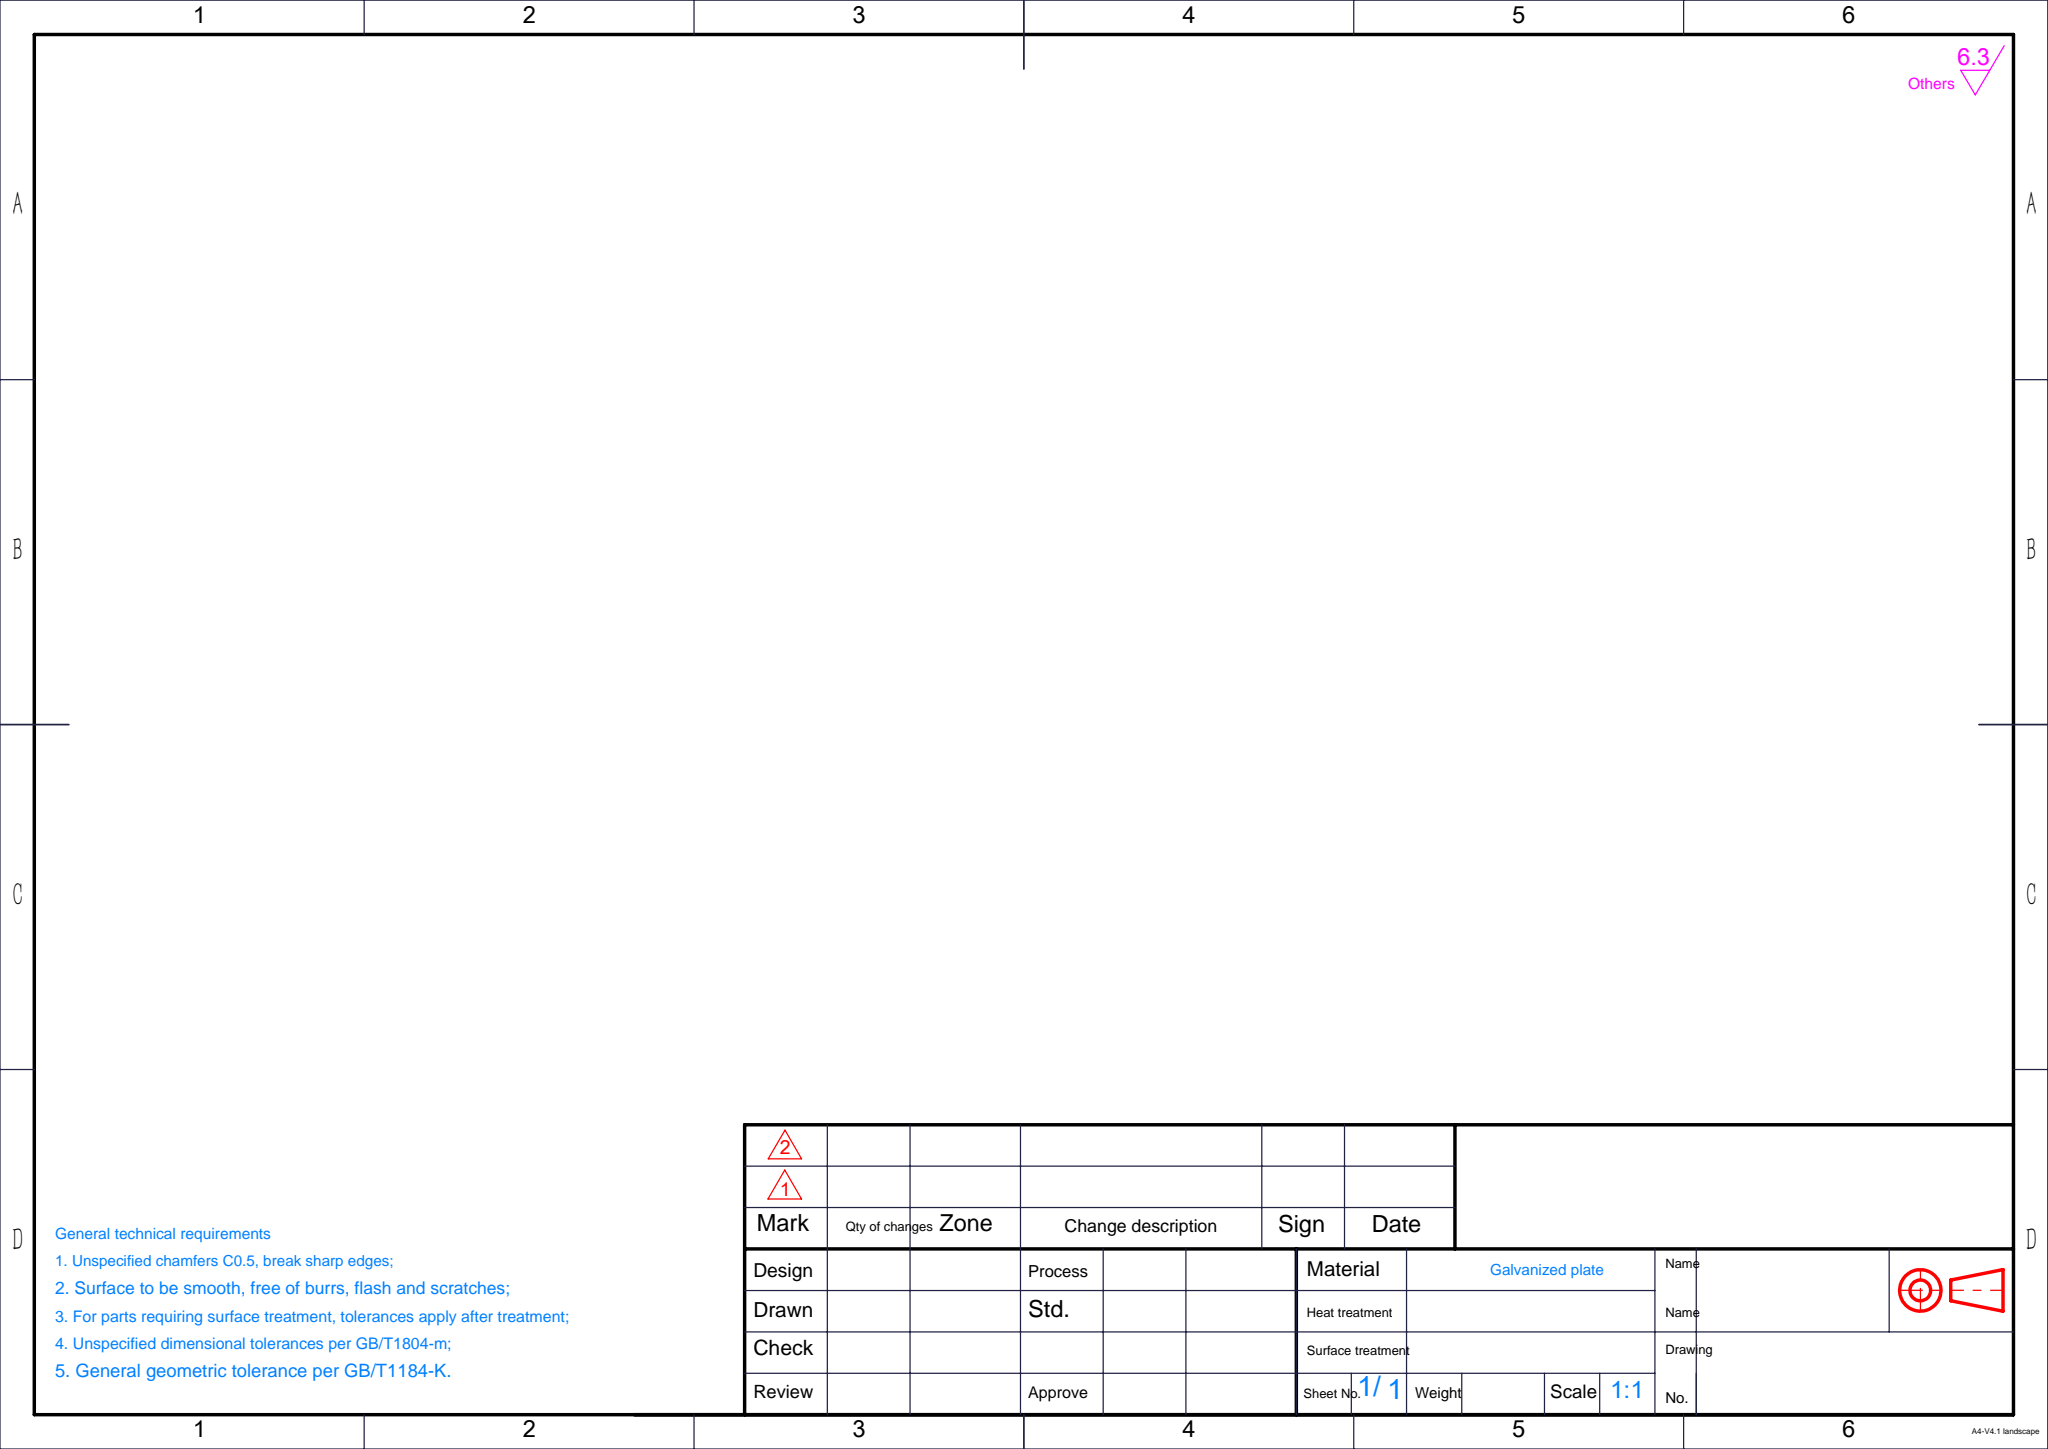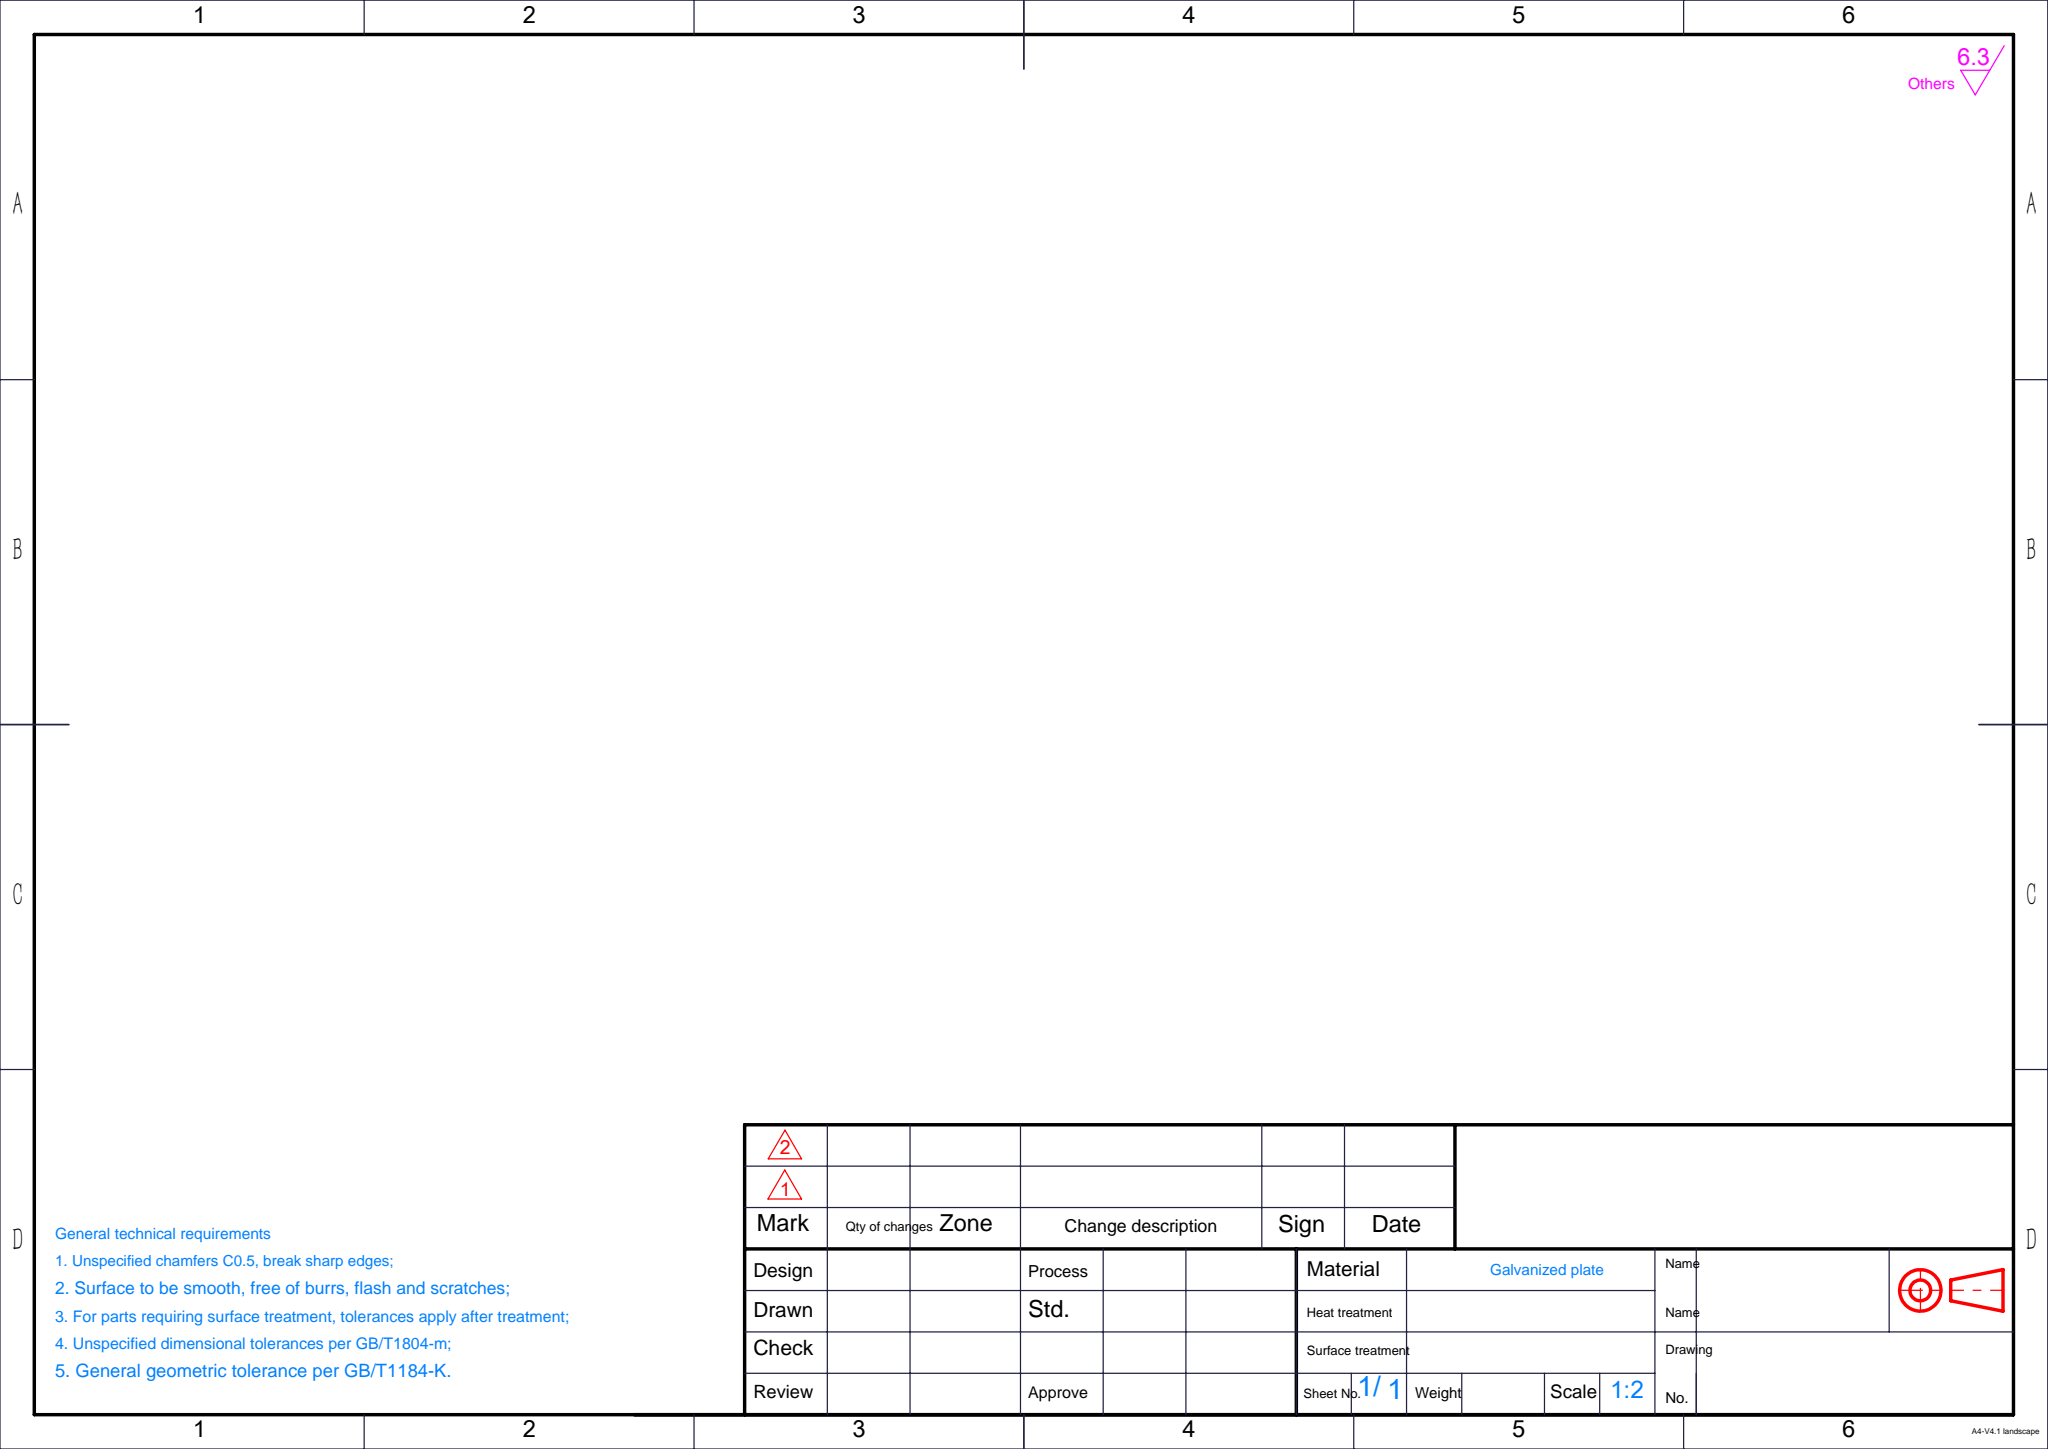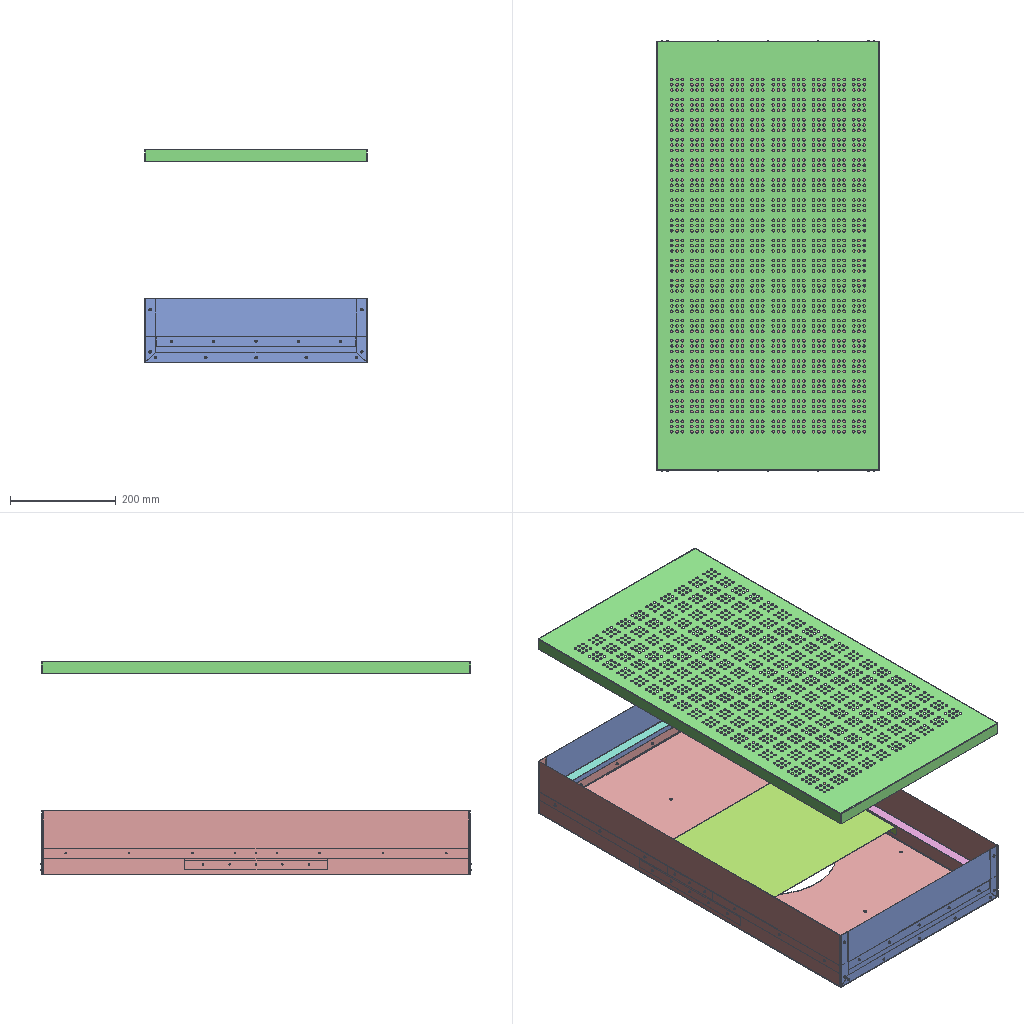Assembly | SolidWorks | 14 different items | 18 placed | box 423 x 814 x 405 mm
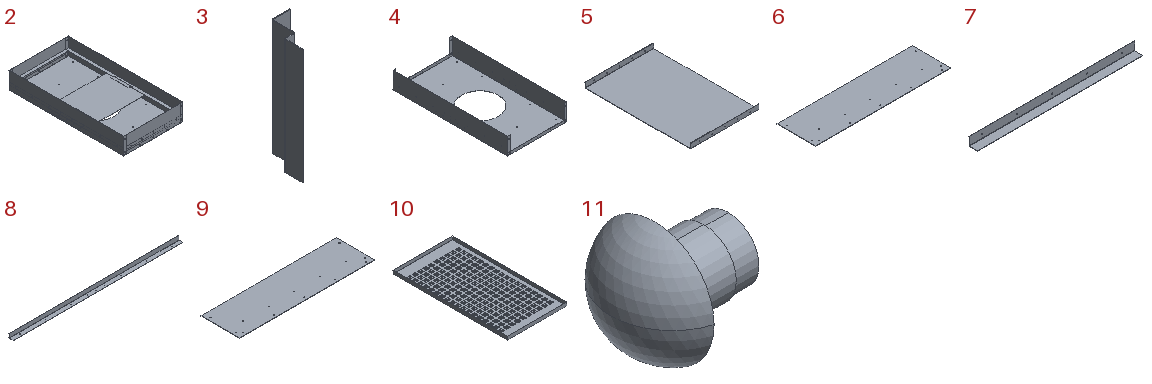Parts list (item | name | quantity | parent item | size | volume | features):
1 | 120 deg blind rivets gb | x1 | - | - | - | -
2 | (subassembly) | x1 | - | 422.6 x 813.6 x 121 mm | 827585 mm3 | features ReferencePattern 29, CompositeCurve 6, MirrorCompFeat 3
3 | - | x2 | in 2 | 30 x 43.6 x 120 mm | 5997 mm3 | features 3DProfileFeature 2, HoleWzd 2, FlatPattern 1, SMBaseFlange 1, SheetMetal 1
4 | - | x1 | in 2 | 420 x 808 x 121 mm | 501647 mm3 | features 3DProfileFeature 5, HoleWzd 5, SketchPattern 4, Chamfer 3, EdgeFlange 2, ICE 2, FlatPattern 1, SMBaseFlange 1, SheetMetal 1
5 | - | x1 | in 2 | 270 x 418 x 20 mm | 147184 mm3 | features 3DProfileFeature 1, EdgeFlange 1, Fillet 1, FlatPattern 1, HoleWzd 1, LPattern 1, MirrorPattern 1, SMBaseFlange 1, SheetMetal 1
6 | - | x1 | - | 420 x 120 x 1 mm | 50337 mm3 | features 3DProfileFeature 1, Chamfer 1, FlatPattern 1, HoleWzd 1, SMBaseFlange 1, SheetMetal 1, SketchPattern 1
7 | - | x2 | in 2 | 378 x 20 x 20 mm | 10260 mm3 | features 3DProfileFeature 1, EdgeFlange 1, FlatPattern 1, HoleWzd 1, LPattern 1, MirrorPattern 1, SMBaseFlange 1, SheetMetal 1
8 | - | x2 | in 2 | 806 x 20 x 20 mm | 21881 mm3 | features 3DProfileFeature 3, HoleWzd 3, EdgeFlange 1, FlatPattern 1, ICE 1, LPattern 1, MirrorPattern 1, SMBaseFlange 1, SheetMetal 1
9 | - | x2 | in 2 | 420 x 120 x 1 mm | 50324 mm3 | features 3DProfileFeature 1, Chamfer 1, FlatPattern 1, HoleWzd 1, ICE 1, SMBaseFlange 1, SheetMetal 1, SketchPattern 1
10 | - | x1 | - | - | 238014 mm3 | features 3DProfileFeature 3, HoleWzd 3, LPattern 3, MirrorPattern 3, EdgeFlange 1, FlatPattern 1, SMBaseFlange 1, SheetMetal 1
11 | - | x1 | - | 4.8 x 4.84 x 4.84 mm | 35.188 mm3 | features Boss 1, RevCut 1, Revolution 1
12 | countersunk head drive rivets gb | x1 | - | - | - | -
13 | rivets for name plate gb | x1 | - | - | - | -
14 | round head rivets gb | x1 | - | - | - | -
Mates (type | each side: item.copy, entity, surface, feature):
In the top assembly
Coincident | 4.1 plane | assembly plane | 3 times
Parallel | 4.1 face plane Base-Flange 1 | 10.1 face plane Base-Flange 1
Parallel | 4.1 face plane Edge-Flange 1 | 10.1 face plane Edge-Flange 1
Coincident | 4.1 face plane Edge-Flange 1 | 10.1 face plane Edge-Flange 1
Coincident | 5.1 plane | assembly plane | 2 times
Coincident | 8.1 plane | assembly plane
Coincident | 7.1 plane | assembly plane
In subassembly 2
Coincident | 4.2 face plane Edge-Flange 1 | 8.2 face plane Base-Flange 1
DistanceDim | 8.2 face plane Edge-Flange 1 | 4.2 face plane Edge-Flange 1
DistanceDim | 5.2 face plane Base-Flange 1 | 4.2 face plane Base-Flange 1
Coincident | 8.2 face plane Edge-Flange 1 | 7.2 face plane Base-Flange 1
Coincident | 8.2 face plane Edge-Flange 1 | 3.1 face plane Base-Flange 1
Coincident | 8.2 face plane Base-Flange 1 | 3.1 face plane Base-Flange 1
Coincident | 9.1 plane | 2.1 plane
Coincident | 4.2 face plane Edge-Flange 2 | 9.1 face plane Base-Flange 1 | 2 times
Coincident | 7.2 plane | 2.1 plane
Coincident | 8.2 plane | 2.1 plane
Coincident | 5.2 plane | 2.1 plane | 2 times
Coincident | 3.1 plane | 2.1 plane
Coincident | 9.1 face plane Base-Flange 1 | 7.2 face plane Edge-Flange 1
Concentric | 4.2 edge | 9.2 edge | 2 times
Coincident | 4.2 face plane Edge-Flange 2 | 9.2 face plane Base-Flange 1